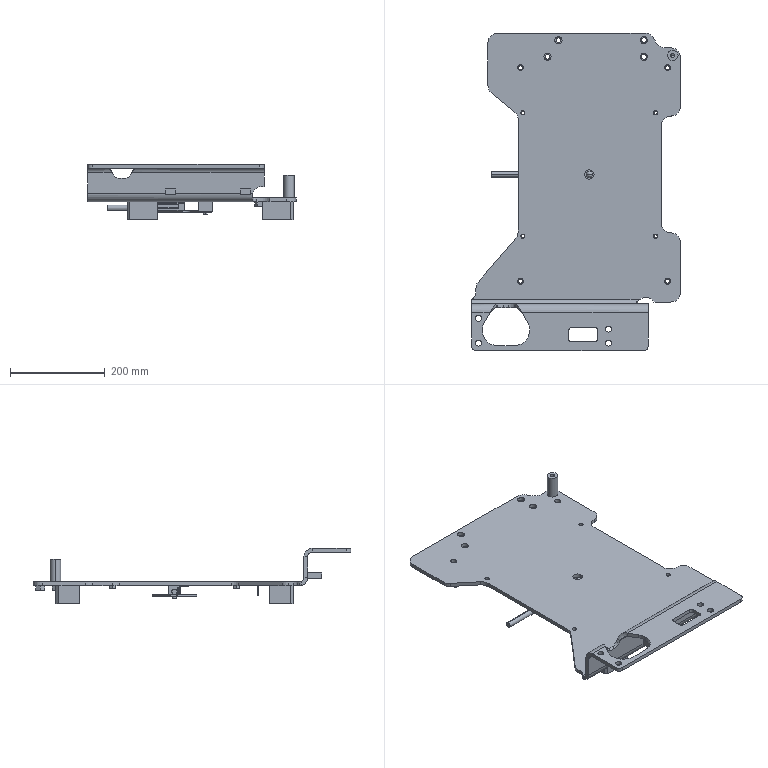Part | SolidWorks | features BaseBody 20 | 20 solids | 321 faces | box 440 x 670 x 117 mm | volume 2554024 mm3 | plane 190 | cylinder 120 | spline 5 | cone 4 | sphere 2 | commonest cylinder face diameters 12.5 x16 40 x15 8.5 x14 9 x10 20 x9 6.75 x8